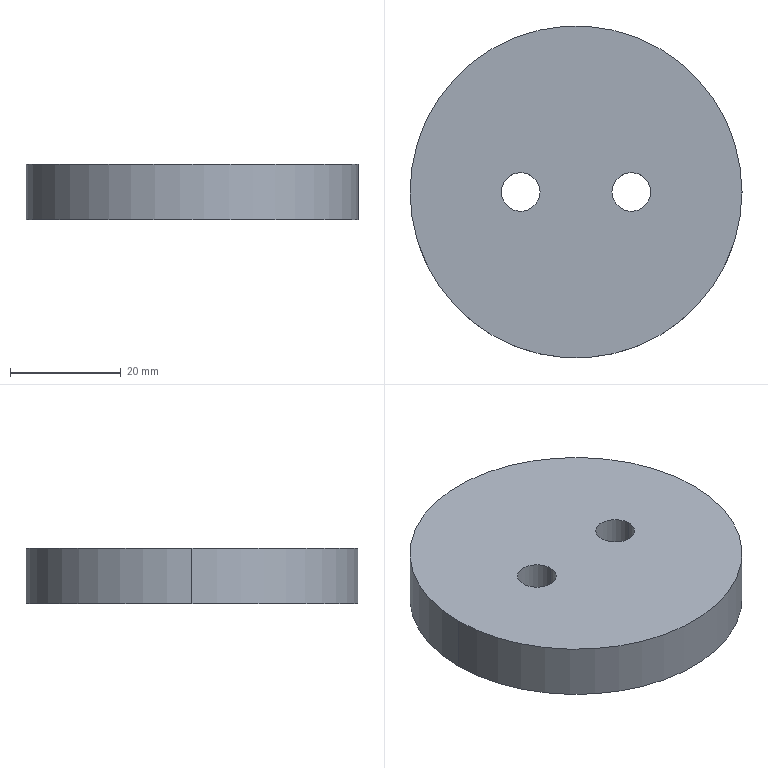Part | STEP file | Single sprocket shaft end cover 1XG | 1 solid | 8 faces | box 60 x 60 x 10 mm | volume 27505 mm3 | cylinder 6 | plane 2 | commonest cylinder face diameters 7 x4 60 x2
STEP:
#1=CARTESIAN_POINT('',(0.,0.,0.));
#2=DIRECTION('',(0.,0.,1.));
#3=DIRECTION('',(1.,0.,0.));
#4=AXIS2_PLACEMENT_3D('',#1,#2,#3);
#5=CARTESIAN_POINT('',(-13.5,0.,10.));
#6=VERTEX_POINT('',#5);
#7=CARTESIAN_POINT('',(-13.5,0.,0.));
#8=VERTEX_POINT('',#7);
#9=CARTESIAN_POINT('',(-13.5,0.,10.));
#10=DIRECTION('',(0.,0.,-1.));
#11=VECTOR('',#10,1.);
#12=LINE('',#9,#11);
#13=CARTESIAN_POINT('',(-10.,0.,10.));
#14=DIRECTION('',(0.,0.,-1.));
#15=DIRECTION('',(-1.,0.,0.));
#16=AXIS2_PLACEMENT_3D('',#13,#14,#15);
#17=CYLINDRICAL_SURFACE('',#16,3.5);
#18=CARTESIAN_POINT('',(6.283,0.));
#19=DIRECTION('',(0.,1.));
#20=VECTOR('',#19,1.);
#21=LINE('',#18,#20);
#22=(GEOMETRIC_REPRESENTATION_CONTEXT(2)PARAMETRIC_REPRESENTATION_CONTEXT()REPRESENTATION_CONTEXT('',''));
#23=DEFINITIONAL_REPRESENTATION('',(#21),#22);
#24=PCURVE('',#17,#23);
#25=CARTESIAN_POINT('',(-10.,0.,10.));
#26=DIRECTION('',(0.,0.,-1.));
#27=DIRECTION('',(-1.,0.,0.));
#28=AXIS2_PLACEMENT_3D('',#25,#26,#27);
#29=CYLINDRICAL_SURFACE('',#28,3.5);
#30=CARTESIAN_POINT('',(0.,0.));
#31=DIRECTION('',(0.,1.));
#32=VECTOR('',#31,1.);
#33=LINE('',#30,#32);
#34=(GEOMETRIC_REPRESENTATION_CONTEXT(2)PARAMETRIC_REPRESENTATION_CONTEXT()REPRESENTATION_CONTEXT('',''));
#35=DEFINITIONAL_REPRESENTATION('',(#33),#34);
#36=PCURVE('',#29,#35);
#37=SURFACE_CURVE('',#12,(#24,#36),.PCURVE_S1.);
#38=EDGE_CURVE('',#6,#8,#37,.T.);
#39=ORIENTED_EDGE('',*,*,#38,.T.);
#40=CARTESIAN_POINT('',(-6.5,0.,0.));
#41=VERTEX_POINT('',#40);
#42=CARTESIAN_POINT('',(-10.,0.,0.));
#43=DIRECTION('',(0.,0.,-1.));
#44=DIRECTION('',(-1.,0.,0.));
#45=AXIS2_PLACEMENT_3D('',#42,#43,#44);
#46=CIRCLE('',#45,3.5);
#47=CARTESIAN_POINT('',(0.,10.));
#48=DIRECTION('',(1.,0.));
#49=VECTOR('',#48,1.);
#50=LINE('',#47,#49);
#51=(GEOMETRIC_REPRESENTATION_CONTEXT(2)PARAMETRIC_REPRESENTATION_CONTEXT()REPRESENTATION_CONTEXT('',''));
#52=DEFINITIONAL_REPRESENTATION('',(#50),#51);
#53=PCURVE('',#17,#52);
#54=CARTESIAN_POINT('',(0.,0.,0.));
#55=DIRECTION('',(0.,0.,1.));
#56=DIRECTION('',(1.,0.,0.));
#57=AXIS2_PLACEMENT_3D('',#54,#55,#56);
#58=PLANE('',#57);
#59=CARTESIAN_POINT('',(-13.5,0.));
#60=CARTESIAN_POINT('',(-13.5,6.062));
#61=CARTESIAN_POINT('',(-8.25,3.031));
#62=CARTESIAN_POINT('',(-3.,0.));
#63=CARTESIAN_POINT('',(-8.25,-3.031));
#64=CARTESIAN_POINT('',(-13.5,-6.062));
#65=CARTESIAN_POINT('',(-13.5,0.));
#66=(BOUNDED_CURVE()B_SPLINE_CURVE(2,(#59,#60,#61,#62,#63,#64,#65),.UNSPECIFIED.,.T.,.F.)B_SPLINE_CURVE_WITH_KNOTS((1,2,2,2,2,1),(-2.094,0.,2.094,4.189,6.283,8.378),.UNSPECIFIED.)CURVE()GEOMETRIC_REPRESENTATION_ITEM()RATIONAL_B_SPLINE_CURVE((1.,0.5,1.,0.5,1.,0.5,1.))REPRESENTATION_ITEM(''));
#67=(GEOMETRIC_REPRESENTATION_CONTEXT(2)PARAMETRIC_REPRESENTATION_CONTEXT()REPRESENTATION_CONTEXT('',''));
#68=DEFINITIONAL_REPRESENTATION('',(#66),#67);
#69=PCURVE('',#58,#68);
#70=SURFACE_CURVE('',#46,(#53,#69),.PCURVE_S1.);
#71=EDGE_CURVE('',#41,#8,#70,.T.);
#72=ORIENTED_EDGE('',*,*,#71,.F.);
#73=CARTESIAN_POINT('',(-6.5,0.,10.));
#74=VERTEX_POINT('',#73);
#75=CARTESIAN_POINT('',(-6.5,0.,10.));
#76=DIRECTION('',(0.,0.,-1.));
#77=VECTOR('',#76,1.);
#78=LINE('',#75,#77);
#79=CARTESIAN_POINT('',(3.142,0.));
#80=DIRECTION('',(0.,1.));
#81=VECTOR('',#80,1.);
#82=LINE('',#79,#81);
#83=(GEOMETRIC_REPRESENTATION_CONTEXT(2)PARAMETRIC_REPRESENTATION_CONTEXT()REPRESENTATION_CONTEXT('',''));
#84=DEFINITIONAL_REPRESENTATION('',(#82),#83);
#85=PCURVE('',#17,#84);
#86=CARTESIAN_POINT('',(3.142,0.));
#87=DIRECTION('',(0.,1.));
#88=VECTOR('',#87,1.);
#89=LINE('',#86,#88);
#90=(GEOMETRIC_REPRESENTATION_CONTEXT(2)PARAMETRIC_REPRESENTATION_CONTEXT()REPRESENTATION_CONTEXT('',''));
#91=DEFINITIONAL_REPRESENTATION('',(#89),#90);
#92=PCURVE('',#29,#91);
#93=SURFACE_CURVE('',#78,(#85,#92),.PCURVE_S1.);
#94=EDGE_CURVE('',#74,#41,#93,.T.);
#95=ORIENTED_EDGE('',*,*,#94,.F.);
#96=CARTESIAN_POINT('',(-10.,0.,10.));
#97=DIRECTION('',(0.,0.,-1.));
#98=DIRECTION('',(-1.,0.,0.));
#99=AXIS2_PLACEMENT_3D('',#96,#97,#98);
#100=CIRCLE('',#99,3.5);
#101=CARTESIAN_POINT('',(0.,0.));
#102=DIRECTION('',(1.,0.));
#103=VECTOR('',#102,1.);
#104=LINE('',#101,#103);
#105=(GEOMETRIC_REPRESENTATION_CONTEXT(2)PARAMETRIC_REPRESENTATION_CONTEXT()REPRESENTATION_CONTEXT('',''));
#106=DEFINITIONAL_REPRESENTATION('',(#104),#105);
#107=PCURVE('',#17,#106);
#108=CARTESIAN_POINT('',(0.,0.,10.));
#109=DIRECTION('',(0.,0.,1.));
#110=DIRECTION('',(1.,0.,0.));
#111=AXIS2_PLACEMENT_3D('',#108,#109,#110);
#112=PLANE('',#111);
#113=CARTESIAN_POINT('',(-13.5,0.));
#114=CARTESIAN_POINT('',(-13.5,6.062));
#115=CARTESIAN_POINT('',(-8.25,3.031));
#116=CARTESIAN_POINT('',(-3.,0.));
#117=CARTESIAN_POINT('',(-8.25,-3.031));
#118=CARTESIAN_POINT('',(-13.5,-6.062));
#119=CARTESIAN_POINT('',(-13.5,0.));
#120=(BOUNDED_CURVE()B_SPLINE_CURVE(2,(#113,#114,#115,#116,#117,#118,#119),.UNSPECIFIED.,.T.,.F.)B_SPLINE_CURVE_WITH_KNOTS((1,2,2,2,2,1),(-2.094,0.,2.094,4.189,6.283,8.378),.UNSPECIFIED.)CURVE()GEOMETRIC_REPRESENTATION_ITEM()RATIONAL_B_SPLINE_CURVE((1.,0.5,1.,0.5,1.,0.5,1.))REPRESENTATION_ITEM(''));
#121=(GEOMETRIC_REPRESENTATION_CONTEXT(2)PARAMETRIC_REPRESENTATION_CONTEXT()REPRESENTATION_CONTEXT('',''));
#122=DEFINITIONAL_REPRESENTATION('',(#120),#121);
#123=PCURVE('',#112,#122);
#124=SURFACE_CURVE('',#100,(#107,#123),.PCURVE_S1.);
#125=EDGE_CURVE('',#74,#6,#124,.T.);
#126=ORIENTED_EDGE('',*,*,#125,.T.);
#127=EDGE_LOOP('',(#39,#72,#95,#126));
#128=FACE_BOUND('',#127,.F.);
#129=ADVANCED_FACE('',(#128),#17,.F.);
#130=CARTESIAN_POINT('',(6.5,0.,10.));
#131=VERTEX_POINT('',#130);
#132=CARTESIAN_POINT('',(6.5,0.,0.));
#133=VERTEX_POINT('',#132);
#134=CARTESIAN_POINT('',(6.5,0.,10.));
#135=DIRECTION('',(0.,0.,-1.));
#136=VECTOR('',#135,1.);
#137=LINE('',#134,#136);
#138=CARTESIAN_POINT('',(10.,0.,10.));
#139=DIRECTION('',(0.,0.,-1.));
#140=DIRECTION('',(-1.,0.,0.));
#141=AXIS2_PLACEMENT_3D('',#138,#139,#140);
#142=CYLINDRICAL_SURFACE('',#141,3.5);
#143=CARTESIAN_POINT('',(6.283,0.));
#144=DIRECTION('',(0.,1.));
#145=VECTOR('',#144,1.);
#146=LINE('',#143,#145);
#147=(GEOMETRIC_REPRESENTATION_CONTEXT(2)PARAMETRIC_REPRESENTATION_CONTEXT()REPRESENTATION_CONTEXT('',''));
#148=DEFINITIONAL_REPRESENTATION('',(#146),#147);
#149=PCURVE('',#142,#148);
#150=CARTESIAN_POINT('',(10.,0.,10.));
#151=DIRECTION('',(0.,0.,-1.));
#152=DIRECTION('',(-1.,0.,0.));
#153=AXIS2_PLACEMENT_3D('',#150,#151,#152);
#154=CYLINDRICAL_SURFACE('',#153,3.5);
#155=CARTESIAN_POINT('',(0.,0.));
#156=DIRECTION('',(0.,1.));
#157=VECTOR('',#156,1.);
#158=LINE('',#155,#157);
#159=(GEOMETRIC_REPRESENTATION_CONTEXT(2)PARAMETRIC_REPRESENTATION_CONTEXT()REPRESENTATION_CONTEXT('',''));
#160=DEFINITIONAL_REPRESENTATION('',(#158),#159);
#161=PCURVE('',#154,#160);
#162=SURFACE_CURVE('',#137,(#149,#161),.PCURVE_S1.);
#163=EDGE_CURVE('',#131,#133,#162,.T.);
#164=ORIENTED_EDGE('',*,*,#163,.T.);
#165=CARTESIAN_POINT('',(13.5,0.,0.));
#166=VERTEX_POINT('',#165);
#167=CARTESIAN_POINT('',(10.,0.,0.));
#168=DIRECTION('',(0.,0.,-1.));
#169=DIRECTION('',(-1.,0.,0.));
#170=AXIS2_PLACEMENT_3D('',#167,#168,#169);
#171=CIRCLE('',#170,3.5);
#172=CARTESIAN_POINT('',(0.,10.));
#173=DIRECTION('',(1.,0.));
#174=VECTOR('',#173,1.);
#175=LINE('',#172,#174);
#176=(GEOMETRIC_REPRESENTATION_CONTEXT(2)PARAMETRIC_REPRESENTATION_CONTEXT()REPRESENTATION_CONTEXT('',''));
#177=DEFINITIONAL_REPRESENTATION('',(#175),#176);
#178=PCURVE('',#142,#177);
#179=CARTESIAN_POINT('',(6.5,0.));
#180=CARTESIAN_POINT('',(6.5,6.062));
#181=CARTESIAN_POINT('',(11.75,3.031));
#182=CARTESIAN_POINT('',(17.,0.));
#183=CARTESIAN_POINT('',(11.75,-3.031));
#184=CARTESIAN_POINT('',(6.5,-6.062));
#185=CARTESIAN_POINT('',(6.5,0.));
#186=(BOUNDED_CURVE()B_SPLINE_CURVE(2,(#179,#180,#181,#182,#183,#184,#185),.UNSPECIFIED.,.T.,.F.)B_SPLINE_CURVE_WITH_KNOTS((1,2,2,2,2,1),(-2.094,0.,2.094,4.189,6.283,8.378),.UNSPECIFIED.)CURVE()GEOMETRIC_REPRESENTATION_ITEM()RATIONAL_B_SPLINE_CURVE((1.,0.5,1.,0.5,1.,0.5,1.))REPRESENTATION_ITEM(''));
#187=(GEOMETRIC_REPRESENTATION_CONTEXT(2)PARAMETRIC_REPRESENTATION_CONTEXT()REPRESENTATION_CONTEXT('',''));
#188=DEFINITIONAL_REPRESENTATION('',(#186),#187);
#189=PCURVE('',#58,#188);
#190=SURFACE_CURVE('',#171,(#178,#189),.PCURVE_S1.);
#191=EDGE_CURVE('',#166,#133,#190,.T.);
#192=ORIENTED_EDGE('',*,*,#191,.F.);
#193=CARTESIAN_POINT('',(13.5,0.,10.));
#194=VERTEX_POINT('',#193);
#195=CARTESIAN_POINT('',(13.5,0.,10.));
#196=DIRECTION('',(0.,0.,-1.));
#197=VECTOR('',#196,1.);
#198=LINE('',#195,#197);
#199=CARTESIAN_POINT('',(3.142,0.));
#200=DIRECTION('',(0.,1.));
#201=VECTOR('',#200,1.);
#202=LINE('',#199,#201);
#203=(GEOMETRIC_REPRESENTATION_CONTEXT(2)PARAMETRIC_REPRESENTATION_CONTEXT()REPRESENTATION_CONTEXT('',''));
#204=DEFINITIONAL_REPRESENTATION('',(#202),#203);
#205=PCURVE('',#142,#204);
#206=CARTESIAN_POINT('',(3.142,0.));
#207=DIRECTION('',(0.,1.));
#208=VECTOR('',#207,1.);
#209=LINE('',#206,#208);
#210=(GEOMETRIC_REPRESENTATION_CONTEXT(2)PARAMETRIC_REPRESENTATION_CONTEXT()REPRESENTATION_CONTEXT('',''));
#211=DEFINITIONAL_REPRESENTATION('',(#209),#210);
#212=PCURVE('',#154,#211);
#213=SURFACE_CURVE('',#198,(#205,#212),.PCURVE_S1.);
#214=EDGE_CURVE('',#194,#166,#213,.T.);
#215=ORIENTED_EDGE('',*,*,#214,.F.);
#216=CARTESIAN_POINT('',(10.,0.,10.));
#217=DIRECTION('',(0.,0.,-1.));
#218=DIRECTION('',(-1.,0.,0.));
#219=AXIS2_PLACEMENT_3D('',#216,#217,#218);
#220=CIRCLE('',#219,3.5);
#221=CARTESIAN_POINT('',(0.,0.));
#222=DIRECTION('',(1.,0.));
#223=VECTOR('',#222,1.);
#224=LINE('',#221,#223);
#225=(GEOMETRIC_REPRESENTATION_CONTEXT(2)PARAMETRIC_REPRESENTATION_CONTEXT()REPRESENTATION_CONTEXT('',''));
#226=DEFINITIONAL_REPRESENTATION('',(#224),#225);
#227=PCURVE('',#142,#226);
#228=CARTESIAN_POINT('',(6.5,0.));
#229=CARTESIAN_POINT('',(6.5,6.062));
#230=CARTESIAN_POINT('',(11.75,3.031));
#231=CARTESIAN_POINT('',(17.,0.));
#232=CARTESIAN_POINT('',(11.75,-3.031));
#233=CARTESIAN_POINT('',(6.5,-6.062));
#234=CARTESIAN_POINT('',(6.5,0.));
#235=(BOUNDED_CURVE()B_SPLINE_CURVE(2,(#228,#229,#230,#231,#232,#233,#234),.UNSPECIFIED.,.T.,.F.)B_SPLINE_CURVE_WITH_KNOTS((1,2,2,2,2,1),(-2.094,0.,2.094,4.189,6.283,8.378),.UNSPECIFIED.)CURVE()GEOMETRIC_REPRESENTATION_ITEM()RATIONAL_B_SPLINE_CURVE((1.,0.5,1.,0.5,1.,0.5,1.))REPRESENTATION_ITEM(''));
#236=(GEOMETRIC_REPRESENTATION_CONTEXT(2)PARAMETRIC_REPRESENTATION_CONTEXT()REPRESENTATION_CONTEXT('',''));
#237=DEFINITIONAL_REPRESENTATION('',(#235),#236);
#238=PCURVE('',#112,#237);
#239=SURFACE_CURVE('',#220,(#227,#238),.PCURVE_S1.);
#240=EDGE_CURVE('',#194,#131,#239,.T.);
#241=ORIENTED_EDGE('',*,*,#240,.T.);
#242=EDGE_LOOP('',(#164,#192,#215,#241));
#243=FACE_BOUND('',#242,.F.);
#244=ADVANCED_FACE('',(#243),#142,.F.);
#245=CARTESIAN_POINT('',(30.,0.,10.));
#246=VERTEX_POINT('',#245);
#247=CARTESIAN_POINT('',(-30.,0.,10.));
#248=VERTEX_POINT('',#247);
#249=CARTESIAN_POINT('',(0.,0.,10.));
#250=DIRECTION('',(0.,0.,1.));
#251=DIRECTION('',(1.,0.,0.));
#252=AXIS2_PLACEMENT_3D('',#249,#250,#251);
#253=CIRCLE('',#252,30.);
#254=CARTESIAN_POINT('',(0.,0.,10.));
#255=DIRECTION('',(0.,0.,-1.));
#256=DIRECTION('',(-1.,0.,0.));
#257=AXIS2_PLACEMENT_3D('',#254,#255,#256);
#258=CYLINDRICAL_SURFACE('',#257,30.);
#259=CARTESIAN_POINT('',(3.142,0.));
#260=DIRECTION('',(-1.,0.));
#261=VECTOR('',#260,1.);
#262=LINE('',#259,#261);
#263=(GEOMETRIC_REPRESENTATION_CONTEXT(2)PARAMETRIC_REPRESENTATION_CONTEXT()REPRESENTATION_CONTEXT('',''));
#264=DEFINITIONAL_REPRESENTATION('',(#262),#263);
#265=PCURVE('',#258,#264);
#266=CARTESIAN_POINT('',(0.,0.));
#267=DIRECTION('',(1.,0.));
#268=AXIS2_PLACEMENT_2D('',#266,#267);
#269=CIRCLE('',#268,30.);
#270=(GEOMETRIC_REPRESENTATION_CONTEXT(2)PARAMETRIC_REPRESENTATION_CONTEXT()REPRESENTATION_CONTEXT('',''));
#271=DEFINITIONAL_REPRESENTATION('',(#269),#270);
#272=PCURVE('',#112,#271);
#273=SURFACE_CURVE('',#253,(#265,#272),.PCURVE_S1.);
#274=EDGE_CURVE('',#246,#248,#273,.T.);
#275=ORIENTED_EDGE('',*,*,#274,.F.);
#276=CARTESIAN_POINT('',(30.,0.,0.));
#277=VERTEX_POINT('',#276);
#278=CARTESIAN_POINT('',(30.,0.,10.));
#279=DIRECTION('',(0.,0.,-1.));
#280=VECTOR('',#279,1.);
#281=LINE('',#278,#280);
#282=CARTESIAN_POINT('',(3.142,0.));
#283=DIRECTION('',(0.,1.));
#284=VECTOR('',#283,1.);
#285=LINE('',#282,#284);
#286=(GEOMETRIC_REPRESENTATION_CONTEXT(2)PARAMETRIC_REPRESENTATION_CONTEXT()REPRESENTATION_CONTEXT('',''));
#287=DEFINITIONAL_REPRESENTATION('',(#285),#286);
#288=PCURVE('',#258,#287);
#289=CARTESIAN_POINT('',(0.,0.,10.));
#290=DIRECTION('',(0.,0.,-1.));
#291=DIRECTION('',(-1.,0.,0.));
#292=AXIS2_PLACEMENT_3D('',#289,#290,#291);
#293=CYLINDRICAL_SURFACE('',#292,30.);
#294=CARTESIAN_POINT('',(3.142,0.));
#295=DIRECTION('',(0.,1.));
#296=VECTOR('',#295,1.);
#297=LINE('',#294,#296);
#298=(GEOMETRIC_REPRESENTATION_CONTEXT(2)PARAMETRIC_REPRESENTATION_CONTEXT()REPRESENTATION_CONTEXT('',''));
#299=DEFINITIONAL_REPRESENTATION('',(#297),#298);
#300=PCURVE('',#293,#299);
#301=SURFACE_CURVE('',#281,(#288,#300),.PCURVE_S1.);
#302=EDGE_CURVE('',#246,#277,#301,.T.);
#303=ORIENTED_EDGE('',*,*,#302,.T.);
#304=CARTESIAN_POINT('',(-30.,0.,0.));
#305=VERTEX_POINT('',#304);
#306=CARTESIAN_POINT('',(0.,0.,0.));
#307=DIRECTION('',(0.,0.,1.));
#308=DIRECTION('',(1.,0.,0.));
#309=AXIS2_PLACEMENT_3D('',#306,#307,#308);
#310=CIRCLE('',#309,30.);
#311=CARTESIAN_POINT('',(3.142,10.));
#312=DIRECTION('',(-1.,0.));
#313=VECTOR('',#312,1.);
#314=LINE('',#311,#313);
#315=(GEOMETRIC_REPRESENTATION_CONTEXT(2)PARAMETRIC_REPRESENTATION_CONTEXT()REPRESENTATION_CONTEXT('',''));
#316=DEFINITIONAL_REPRESENTATION('',(#314),#315);
#317=PCURVE('',#258,#316);
#318=CARTESIAN_POINT('',(0.,0.));
#319=DIRECTION('',(1.,0.));
#320=AXIS2_PLACEMENT_2D('',#318,#319);
#321=CIRCLE('',#320,30.);
#322=(GEOMETRIC_REPRESENTATION_CONTEXT(2)PARAMETRIC_REPRESENTATION_CONTEXT()REPRESENTATION_CONTEXT('',''));
#323=DEFINITIONAL_REPRESENTATION('',(#321),#322);
#324=PCURVE('',#58,#323);
#325=SURFACE_CURVE('',#310,(#317,#324),.PCURVE_S1.);
#326=EDGE_CURVE('',#277,#305,#325,.T.);
#327=ORIENTED_EDGE('',*,*,#326,.T.);
#328=CARTESIAN_POINT('',(-30.,0.,10.));
#329=DIRECTION('',(0.,0.,-1.));
#330=VECTOR('',#329,1.);
#331=LINE('',#328,#330);
#332=CARTESIAN_POINT('',(0.,0.));
#333=DIRECTION('',(0.,1.));
#334=VECTOR('',#333,1.);
#335=LINE('',#332,#334);
#336=(GEOMETRIC_REPRESENTATION_CONTEXT(2)PARAMETRIC_REPRESENTATION_CONTEXT()REPRESENTATION_CONTEXT('',''));
#337=DEFINITIONAL_REPRESENTATION('',(#335),#336);
#338=PCURVE('',#258,#337);
#339=CARTESIAN_POINT('',(6.283,0.));
#340=DIRECTION('',(0.,1.));
#341=VECTOR('',#340,1.);
#342=LINE('',#339,#341);
#343=(GEOMETRIC_REPRESENTATION_CONTEXT(2)PARAMETRIC_REPRESENTATION_CONTEXT()REPRESENTATION_CONTEXT('',''));
#344=DEFINITIONAL_REPRESENTATION('',(#342),#343);
#345=PCURVE('',#293,#344);
#346=SURFACE_CURVE('',#331,(#338,#345),.PCURVE_S1.);
#347=EDGE_CURVE('',#248,#305,#346,.T.);
#348=ORIENTED_EDGE('',*,*,#347,.F.);
#349=EDGE_LOOP('',(#275,#303,#327,#348));
#350=FACE_BOUND('',#349,.T.);
#351=ADVANCED_FACE('',(#350),#258,.T.);
#352=ORIENTED_EDGE('',*,*,#302,.F.);
#353=CARTESIAN_POINT('',(0.,0.,10.));
#354=DIRECTION('',(0.,0.,1.));
#355=DIRECTION('',(1.,0.,0.));
#356=AXIS2_PLACEMENT_3D('',#353,#354,#355);
#357=CIRCLE('',#356,30.);
#358=CARTESIAN_POINT('',(9.425,0.));
#359=DIRECTION('',(-1.,0.));
#360=VECTOR('',#359,1.);
#361=LINE('',#358,#360);
#362=(GEOMETRIC_REPRESENTATION_CONTEXT(2)PARAMETRIC_REPRESENTATION_CONTEXT()REPRESENTATION_CONTEXT('',''));
#363=DEFINITIONAL_REPRESENTATION('',(#361),#362);
#364=PCURVE('',#293,#363);
#365=CARTESIAN_POINT('',(0.,0.));
#366=DIRECTION('',(1.,0.));
#367=AXIS2_PLACEMENT_2D('',#365,#366);
#368=CIRCLE('',#367,30.);
#369=(GEOMETRIC_REPRESENTATION_CONTEXT(2)PARAMETRIC_REPRESENTATION_CONTEXT()REPRESENTATION_CONTEXT('',''));
#370=DEFINITIONAL_REPRESENTATION('',(#368),#369);
#371=PCURVE('',#112,#370);
#372=SURFACE_CURVE('',#357,(#364,#371),.PCURVE_S1.);
#373=EDGE_CURVE('',#248,#246,#372,.T.);
#374=ORIENTED_EDGE('',*,*,#373,.F.);
#375=ORIENTED_EDGE('',*,*,#347,.T.);
#376=CARTESIAN_POINT('',(0.,0.,0.));
#377=DIRECTION('',(0.,0.,1.));
#378=DIRECTION('',(1.,0.,0.));
#379=AXIS2_PLACEMENT_3D('',#376,#377,#378);
#380=CIRCLE('',#379,30.);
#381=CARTESIAN_POINT('',(9.425,10.));
#382=DIRECTION('',(-1.,0.));
#383=VECTOR('',#382,1.);
#384=LINE('',#381,#383);
#385=(GEOMETRIC_REPRESENTATION_CONTEXT(2)PARAMETRIC_REPRESENTATION_CONTEXT()REPRESENTATION_CONTEXT('',''));
#386=DEFINITIONAL_REPRESENTATION('',(#384),#385);
#387=PCURVE('',#293,#386);
#388=CARTESIAN_POINT('',(0.,0.));
#389=DIRECTION('',(1.,0.));
#390=AXIS2_PLACEMENT_2D('',#388,#389);
#391=CIRCLE('',#390,30.);
#392=(GEOMETRIC_REPRESENTATION_CONTEXT(2)PARAMETRIC_REPRESENTATION_CONTEXT()REPRESENTATION_CONTEXT('',''));
#393=DEFINITIONAL_REPRESENTATION('',(#391),#392);
#394=PCURVE('',#58,#393);
#395=SURFACE_CURVE('',#380,(#387,#394),.PCURVE_S1.);
#396=EDGE_CURVE('',#305,#277,#395,.T.);
#397=ORIENTED_EDGE('',*,*,#396,.T.);
#398=EDGE_LOOP('',(#352,#374,#375,#397));
#399=FACE_BOUND('',#398,.T.);
#400=ADVANCED_FACE('',(#399),#293,.T.);
#401=CARTESIAN_POINT('',(-10.,0.,10.));
#402=DIRECTION('',(0.,0.,-1.));
#403=DIRECTION('',(-1.,0.,0.));
#404=AXIS2_PLACEMENT_3D('',#401,#402,#403);
#405=CIRCLE('',#404,3.5);
#406=CARTESIAN_POINT('',(-13.5,0.));
#407=CARTESIAN_POINT('',(-13.5,6.062));
#408=CARTESIAN_POINT('',(-8.25,3.031));
#409=CARTESIAN_POINT('',(-3.,0.));
#410=CARTESIAN_POINT('',(-8.25,-3.031));
#411=CARTESIAN_POINT('',(-13.5,-6.062));
#412=CARTESIAN_POINT('',(-13.5,0.));
#413=(BOUNDED_CURVE()B_SPLINE_CURVE(2,(#406,#407,#408,#409,#410,#411,#412),.UNSPECIFIED.,.T.,.F.)B_SPLINE_CURVE_WITH_KNOTS((1,2,2,2,2,1),(-2.094,0.,2.094,4.189,6.283,8.378),.UNSPECIFIED.)CURVE()GEOMETRIC_REPRESENTATION_ITEM()RATIONAL_B_SPLINE_CURVE((1.,0.5,1.,0.5,1.,0.5,1.))REPRESENTATION_ITEM(''));
#414=(GEOMETRIC_REPRESENTATION_CONTEXT(2)PARAMETRIC_REPRESENTATION_CONTEXT()REPRESENTATION_CONTEXT('',''));
#415=DEFINITIONAL_REPRESENTATION('',(#413),#414);
#416=PCURVE('',#112,#415);
#417=CARTESIAN_POINT('',(0.,0.));
#418=DIRECTION('',(1.,0.));
#419=VECTOR('',#418,1.);
#420=LINE('',#417,#419);
#421=(GEOMETRIC_REPRESENTATION_CONTEXT(2)PARAMETRIC_REPRESENTATION_CONTEXT()REPRESENTATION_CONTEXT('',''));
#422=DEFINITIONAL_REPRESENTATION('',(#420),#421);
#423=PCURVE('',#29,#422);
#424=SURFACE_CURVE('',#405,(#416,#423),.PCURVE_S1.);
#425=EDGE_CURVE('',#6,#74,#424,.T.);
#426=ORIENTED_EDGE('',*,*,#425,.T.);
#427=ORIENTED_EDGE('',*,*,#125,.T.);
#428=EDGE_LOOP('',(#426,#427));
#429=FACE_BOUND('',#428,.T.);
#430=CARTESIAN_POINT('',(10.,0.,10.));
#431=DIRECTION('',(0.,0.,-1.));
#432=DIRECTION('',(-1.,0.,0.));
#433=AXIS2_PLACEMENT_3D('',#430,#431,#432);
#434=CIRCLE('',#433,3.5);
#435=CARTESIAN_POINT('',(6.5,0.));
#436=CARTESIAN_POINT('',(6.5,6.062));
#437=CARTESIAN_POINT('',(11.75,3.031));
#438=CARTESIAN_POINT('',(17.,0.));
#439=CARTESIAN_POINT('',(11.75,-3.031));
#440=CARTESIAN_POINT('',(6.5,-6.062));
#441=CARTESIAN_POINT('',(6.5,0.));
#442=(BOUNDED_CURVE()B_SPLINE_CURVE(2,(#435,#436,#437,#438,#439,#440,#441),.UNSPECIFIED.,.T.,.F.)B_SPLINE_CURVE_WITH_KNOTS((1,2,2,2,2,1),(-2.094,0.,2.094,4.189,6.283,8.378),.UNSPECIFIED.)CURVE()GEOMETRIC_REPRESENTATION_ITEM()RATIONAL_B_SPLINE_CURVE((1.,0.5,1.,0.5,1.,0.5,1.))REPRESENTATION_ITEM(''));
#443=(GEOMETRIC_REPRESENTATION_CONTEXT(2)PARAMETRIC_REPRESENTATION_CONTEXT()REPRESENTATION_CONTEXT('',''));
#444=DEFINITIONAL_REPRESENTATION('',(#442),#443);
#445=PCURVE('',#112,#444);
#446=CARTESIAN_POINT('',(0.,0.));
#447=DIRECTION('',(1.,0.));
#448=VECTOR('',#447,1.);
#449=LINE('',#446,#448);
#450=(GEOMETRIC_REPRESENTATION_CONTEXT(2)PARAMETRIC_REPRESENTATION_CONTEXT()REPRESENTATION_CONTEXT('',''));
#451=DEFINITIONAL_REPRESENTATION('',(#449),#450);
#452=PCURVE('',#154,#451);
#453=SURFACE_CURVE('',#434,(#445,#452),.PCURVE_S1.);
#454=EDGE_CURVE('',#131,#194,#453,.T.);
#455=ORIENTED_EDGE('',*,*,#454,.T.);
#456=ORIENTED_EDGE('',*,*,#240,.T.);
#457=EDGE_LOOP('',(#455,#456));
#458=FACE_BOUND('',#457,.T.);
#459=ORIENTED_EDGE('',*,*,#373,.T.);
#460=ORIENTED_EDGE('',*,*,#274,.T.);
#461=EDGE_LOOP('',(#459,#460));
#462=FACE_BOUND('',#461,.T.);
#463=ADVANCED_FACE('',(#429,#458,#462),#112,.T.);
#464=CARTESIAN_POINT('',(-10.,0.,0.));
#465=DIRECTION('',(0.,0.,-1.));
#466=DIRECTION('',(-1.,0.,0.));
#467=AXIS2_PLACEMENT_3D('',#464,#465,#466);
#468=CIRCLE('',#467,3.5);
#469=CARTESIAN_POINT('',(-13.5,0.));
#470=CARTESIAN_POINT('',(-13.5,6.062));
#471=CARTESIAN_POINT('',(-8.25,3.031));
#472=CARTESIAN_POINT('',(-3.,0.));
#473=CARTESIAN_POINT('',(-8.25,-3.031));
#474=CARTESIAN_POINT('',(-13.5,-6.062));
#475=CARTESIAN_POINT('',(-13.5,0.));
#476=(BOUNDED_CURVE()B_SPLINE_CURVE(2,(#469,#470,#471,#472,#473,#474,#475),.UNSPECIFIED.,.T.,.F.)B_SPLINE_CURVE_WITH_KNOTS((1,2,2,2,2,1),(-2.094,0.,2.094,4.189,6.283,8.378),.UNSPECIFIED.)CURVE()GEOMETRIC_REPRESENTATION_ITEM()RATIONAL_B_SPLINE_CURVE((1.,0.5,1.,0.5,1.,0.5,1.))REPRESENTATION_ITEM(''));
#477=(GEOMETRIC_REPRESENTATION_CONTEXT(2)PARAMETRIC_REPRESENTATION_CONTEXT()REPRESENTATION_CONTEXT('',''));
#478=DEFINITIONAL_REPRESENTATION('',(#476),#477);
#479=PCURVE('',#58,#478);
#480=CARTESIAN_POINT('',(0.,10.));
#481=DIRECTION('',(1.,0.));
#482=VECTOR('',#481,1.);
#483=LINE('',#480,#482);
#484=(GEOMETRIC_REPRESENTATION_CONTEXT(2)PARAMETRIC_REPRESENTATION_CONTEXT()REPRESENTATION_CONTEXT('',''));
#485=DEFINITIONAL_REPRESENTATION('',(#483),#484);
#486=PCURVE('',#29,#485);
#487=SURFACE_CURVE('',#468,(#479,#486),.PCURVE_S1.);
#488=EDGE_CURVE('',#8,#41,#487,.T.);
#489=ORIENTED_EDGE('',*,*,#488,.F.);
#490=ORIENTED_EDGE('',*,*,#71,.F.);
#491=EDGE_LOOP('',(#489,#490));
#492=FACE_BOUND('',#491,.T.);
#493=CARTESIAN_POINT('',(10.,0.,0.));
#494=DIRECTION('',(0.,0.,-1.));
#495=DIRECTION('',(-1.,0.,0.));
#496=AXIS2_PLACEMENT_3D('',#493,#494,#495);
#497=CIRCLE('',#496,3.5);
#498=CARTESIAN_POINT('',(6.5,0.));
#499=CARTESIAN_POINT('',(6.5,6.062));
#500=CARTESIAN_POINT('',(11.75,3.031));
#501=CARTESIAN_POINT('',(17.,0.));
#502=CARTESIAN_POINT('',(11.75,-3.031));
#503=CARTESIAN_POINT('',(6.5,-6.062));
#504=CARTESIAN_POINT('',(6.5,0.));
#505=(BOUNDED_CURVE()B_SPLINE_CURVE(2,(#498,#499,#500,#501,#502,#503,#504),.UNSPECIFIED.,.T.,.F.)B_SPLINE_CURVE_WITH_KNOTS((1,2,2,2,2,1),(-2.094,0.,2.094,4.189,6.283,8.378),.UNSPECIFIED.)CURVE()GEOMETRIC_REPRESENTATION_ITEM()RATIONAL_B_SPLINE_CURVE((1.,0.5,1.,0.5,1.,0.5,1.))REPRESENTATION_ITEM(''));
#506=(GEOMETRIC_REPRESENTATION_CONTEXT(2)PARAMETRIC_REPRESENTATION_CONTEXT()REPRESENTATION_CONTEXT('',''));
#507=DEFINITIONAL_REPRESENTATION('',(#505),#506);
#508=PCURVE('',#58,#507);
#509=CARTESIAN_POINT('',(0.,10.));
#510=DIRECTION('',(1.,0.));
#511=VECTOR('',#510,1.);
#512=LINE('',#509,#511);
#513=(GEOMETRIC_REPRESENTATION_CONTEXT(2)PARAMETRIC_REPRESENTATION_CONTEXT()REPRESENTATION_CONTEXT('',''));
#514=DEFINITIONAL_REPRESENTATION('',(#512),#513);
#515=PCURVE('',#154,#514);
#516=SURFACE_CURVE('',#497,(#508,#515),.PCURVE_S1.);
#517=EDGE_CURVE('',#133,#166,#516,.T.);
#518=ORIENTED_EDGE('',*,*,#517,.F.);
#519=ORIENTED_EDGE('',*,*,#191,.F.);
#520=EDGE_LOOP('',(#518,#519));
#521=FACE_BOUND('',#520,.T.);
#522=ORIENTED_EDGE('',*,*,#396,.F.);
#523=ORIENTED_EDGE('',*,*,#326,.F.);
#524=EDGE_LOOP('',(#522,#523));
#525=FACE_BOUND('',#524,.T.);
#526=ADVANCED_FACE('',(#492,#521,#525),#58,.F.);
#527=ORIENTED_EDGE('',*,*,#517,.F.);
#528=ORIENTED_EDGE('',*,*,#163,.F.);
#529=ORIENTED_EDGE('',*,*,#454,.T.);
#530=ORIENTED_EDGE('',*,*,#214,.T.);
#531=EDGE_LOOP('',(#527,#528,#529,#530));
#532=FACE_BOUND('',#531,.F.);
#533=ADVANCED_FACE('',(#532),#154,.F.);
#534=ORIENTED_EDGE('',*,*,#488,.F.);
#535=ORIENTED_EDGE('',*,*,#38,.F.);
#536=ORIENTED_EDGE('',*,*,#425,.T.);
#537=ORIENTED_EDGE('',*,*,#94,.T.);
#538=EDGE_LOOP('',(#534,#535,#536,#537));
#539=FACE_BOUND('',#538,.F.);
#540=ADVANCED_FACE('',(#539),#29,.F.);
#541=CLOSED_SHELL('',(#129,#244,#351,#400,#463,#526,#533,#540));
#542=MANIFOLD_SOLID_BREP('',#541);
#543=(LENGTH_UNIT()NAMED_UNIT(*)SI_UNIT(.MILLI.,.METRE.));
#544=UNCERTAINTY_MEASURE_WITH_UNIT(LENGTH_MEASURE(0.0000001),#543,'','');
#545=(NAMED_UNIT(*)PLANE_ANGLE_UNIT()SI_UNIT($,.RADIAN.));
#546=(NAMED_UNIT(*)SI_UNIT($,.STERADIAN.)SOLID_ANGLE_UNIT());
#547=(GEOMETRIC_REPRESENTATION_CONTEXT(3)GLOBAL_UNCERTAINTY_ASSIGNED_CONTEXT((#544))GLOBAL_UNIT_ASSIGNED_CONTEXT((#543,#545,#546))REPRESENTATION_CONTEXT('',''));
#548=ADVANCED_BREP_SHAPE_REPRESENTATION('',(#4,#542),#547);